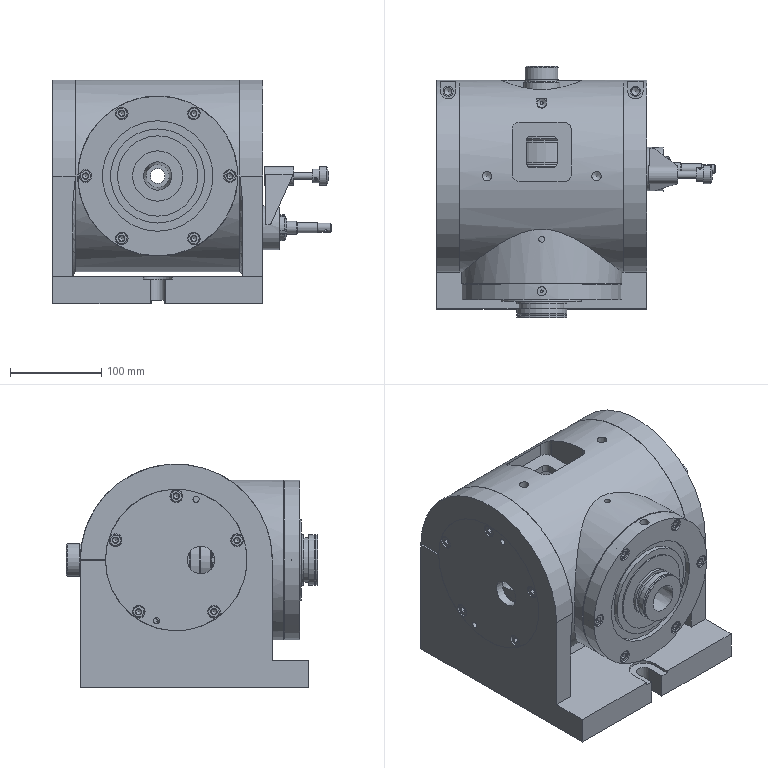Part | NX | features META 246, BREP 240, DATUM_CSYS 113, SKETCH 91, EXTRUDE 77, SYMBOLIC_THREAD 42, SIMPLE HOLE 28, HOLE PACKAGE 26, IDENTICAL INSTANCE OUTPUT 24, CHAMFER 22, Instance Feature 22, BLEND 17, SWP104 15, CBORE_HOLE 8, INSTANCE 8, DATUM_PLANE 6, EXTRACT_STRING 6, MASTER SNAPSHOT BODY 6, REPLACE_FACE 6, Pattern Feature 5, SUBTRACT 5, FSET 4, LINE 4, THREADS 4, UNITE 4, CIRCULAR_ISET 2, CYLINDER 2, FACE_BLEND 2, Mirror Feature 2, Pattern Face Feature 2, SKIN 2, TRANSFORM_ISET 2, ASSOCIATIVE_INTERSECTION 1, CSUNK_HOLE 1, Container 1, DELETE FACE 1, EXTRACT_BODY 1, Geometry Instance 1, HELIX 1, INTERSECT 1, OFFSET_REGION 1, SPLIT BODY 1, TRIM BODY 1 | 48 solids | 5057 faces | volume 7825031 mm3 | spline 3034 | cylinder 1064 | plane 579 | cone 258 | torus 117 | sphere 5 | commonest cylinder face diameters 115.5 x472 119.5 x122 96 x120 10 x39 6.8 x26 14 x22